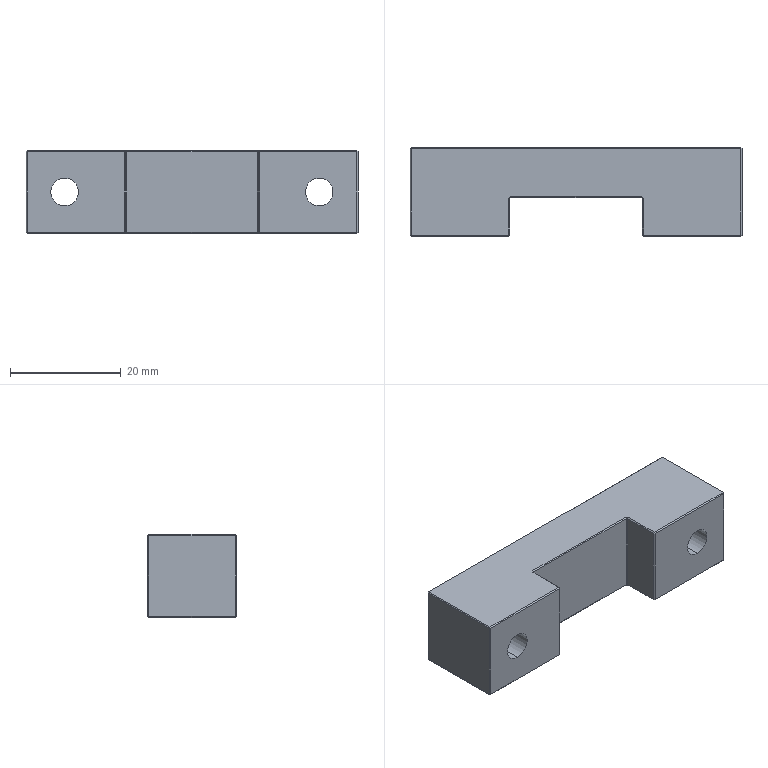Part | 1 solid | 58 faces | box 60 x 16 x 15 mm | volume 11243 mm3 | plane 50 | cone 4 | cylinder 4 | commonest cylinder face diameters 5 x4
STEP:
#1=CARTESIAN_POINT('',(22.997,-0.2,5.));
#2=VERTEX_POINT('',#1);
#3=CARTESIAN_POINT('',(22.997,-0.2,10.));
#4=VERTEX_POINT('',#3);
#5=CARTESIAN_POINT('',(22.997,-0.2,7.5));
#6=DIRECTION('',(0.,1.,0.));
#7=DIRECTION('',(0.,0.,-1.));
#8=AXIS2_PLACEMENT_3D('',#5,#6,#7);
#9=CIRCLE('',#8,2.5);
#10=EDGE_CURVE('',#2,#4,#9,.T.);
#11=ORIENTED_EDGE('',*,*,#10,.F.);
#12=CARTESIAN_POINT('',(22.997,0.,4.8));
#13=VERTEX_POINT('',#12);
#14=CARTESIAN_POINT('',(22.997,0.,4.8));
#15=DIRECTION('',(0.,0.7071,-0.7071));
#16=VECTOR('',#15,1000.);
#17=LINE('',#14,#16);
#18=EDGE_CURVE('',#2,#13,#17,.T.);
#19=ORIENTED_EDGE('',*,*,#18,.T.);
#20=CARTESIAN_POINT('',(22.997,0.,10.2));
#21=VERTEX_POINT('',#20);
#22=CARTESIAN_POINT('',(22.997,0.,7.5));
#23=DIRECTION('',(0.,-1.,0.));
#24=DIRECTION('',(1.,0.,0.));
#25=AXIS2_PLACEMENT_3D('',#22,#23,#24);
#26=CIRCLE('',#25,2.7);
#27=EDGE_CURVE('',#21,#13,#26,.T.);
#28=ORIENTED_EDGE('',*,*,#27,.F.);
#29=CARTESIAN_POINT('',(22.997,0.,10.2));
#30=DIRECTION('',(0.,0.7071,0.7071));
#31=VECTOR('',#30,1000.);
#32=LINE('',#29,#31);
#33=EDGE_CURVE('',#4,#21,#32,.T.);
#34=ORIENTED_EDGE('',*,*,#33,.F.);
#35=EDGE_LOOP('',(#11,#19,#28,#34));
#36=FACE_OUTER_BOUND('',#35,.T.);
#37=CARTESIAN_POINT('',(22.997,0.,7.5));
#38=DIRECTION('',(0.,1.,0.));
#39=DIRECTION('',(0.,0.,1.));
#40=AXIS2_PLACEMENT_3D('',#37,#38,#39);
#41=CONICAL_SURFACE('',#40,2.7,0.7854);
#42=ADVANCED_FACE('',(#36),#41,.F.);
#43=CARTESIAN_POINT('',(-23.003,-0.2,5.));
#44=VERTEX_POINT('',#43);
#45=CARTESIAN_POINT('',(-23.003,-0.2,10.));
#46=VERTEX_POINT('',#45);
#47=CARTESIAN_POINT('',(-23.003,-0.2,7.5));
#48=DIRECTION('',(0.,1.,0.));
#49=DIRECTION('',(0.,0.,-1.));
#50=AXIS2_PLACEMENT_3D('',#47,#48,#49);
#51=CIRCLE('',#50,2.5);
#52=EDGE_CURVE('',#44,#46,#51,.T.);
#53=ORIENTED_EDGE('',*,*,#52,.F.);
#54=CARTESIAN_POINT('',(-23.003,0.,4.8));
#55=VERTEX_POINT('',#54);
#56=CARTESIAN_POINT('',(-23.003,0.,4.8));
#57=DIRECTION('',(0.,0.7071,-0.7071));
#58=VECTOR('',#57,1000.);
#59=LINE('',#56,#58);
#60=EDGE_CURVE('',#44,#55,#59,.T.);
#61=ORIENTED_EDGE('',*,*,#60,.T.);
#62=CARTESIAN_POINT('',(-23.003,0.,10.2));
#63=VERTEX_POINT('',#62);
#64=CARTESIAN_POINT('',(-23.003,0.,7.5));
#65=DIRECTION('',(0.,-1.,0.));
#66=DIRECTION('',(1.,0.,0.));
#67=AXIS2_PLACEMENT_3D('',#64,#65,#66);
#68=CIRCLE('',#67,2.7);
#69=EDGE_CURVE('',#63,#55,#68,.T.);
#70=ORIENTED_EDGE('',*,*,#69,.F.);
#71=CARTESIAN_POINT('',(-23.003,0.,10.2));
#72=DIRECTION('',(0.,0.7071,0.7071));
#73=VECTOR('',#72,1000.);
#74=LINE('',#71,#73);
#75=EDGE_CURVE('',#46,#63,#74,.T.);
#76=ORIENTED_EDGE('',*,*,#75,.F.);
#77=EDGE_LOOP('',(#53,#61,#70,#76));
#78=FACE_OUTER_BOUND('',#77,.T.);
#79=CARTESIAN_POINT('',(-23.003,0.,7.5));
#80=DIRECTION('',(0.,1.,0.));
#81=DIRECTION('',(0.,0.,1.));
#82=AXIS2_PLACEMENT_3D('',#79,#80,#81);
#83=CONICAL_SURFACE('',#82,2.7,0.7854);
#84=ADVANCED_FACE('',(#78),#83,.F.);
#85=ORIENTED_EDGE('',*,*,#52,.T.);
#86=CARTESIAN_POINT('',(-23.003,-16.,10.));
#87=VERTEX_POINT('',#86);
#88=CARTESIAN_POINT('',(-23.003,-16.,10.));
#89=DIRECTION('',(0.,-1.,0.));
#90=VECTOR('',#89,1000.);
#91=LINE('',#88,#90);
#92=EDGE_CURVE('',#46,#87,#91,.T.);
#93=ORIENTED_EDGE('',*,*,#92,.T.);
#94=CARTESIAN_POINT('',(-23.003,-16.,5.));
#95=VERTEX_POINT('',#94);
#96=CARTESIAN_POINT('',(-23.003,-16.,7.5));
#97=DIRECTION('',(0.,-1.,0.));
#98=DIRECTION('',(0.,0.,-1.));
#99=AXIS2_PLACEMENT_3D('',#96,#97,#98);
#100=CIRCLE('',#99,2.5);
#101=EDGE_CURVE('',#87,#95,#100,.T.);
#102=ORIENTED_EDGE('',*,*,#101,.T.);
#103=CARTESIAN_POINT('',(-23.003,-16.,5.));
#104=DIRECTION('',(0.,-1.,0.));
#105=VECTOR('',#104,1000.);
#106=LINE('',#103,#105);
#107=EDGE_CURVE('',#44,#95,#106,.T.);
#108=ORIENTED_EDGE('',*,*,#107,.F.);
#109=EDGE_LOOP('',(#85,#93,#102,#108));
#110=FACE_OUTER_BOUND('',#109,.T.);
#111=CARTESIAN_POINT('',(-23.003,-16.,7.5));
#112=DIRECTION('',(0.,-1.,0.));
#113=DIRECTION('',(0.,0.,-1.));
#114=AXIS2_PLACEMENT_3D('',#111,#112,#113);
#115=CYLINDRICAL_SURFACE('',#114,2.5);
#116=ADVANCED_FACE('',(#110),#115,.F.);
#117=ORIENTED_EDGE('',*,*,#10,.T.);
#118=CARTESIAN_POINT('',(22.997,-16.,10.));
#119=VERTEX_POINT('',#118);
#120=CARTESIAN_POINT('',(22.997,-16.,10.));
#121=DIRECTION('',(0.,-1.,0.));
#122=VECTOR('',#121,1000.);
#123=LINE('',#120,#122);
#124=EDGE_CURVE('',#4,#119,#123,.T.);
#125=ORIENTED_EDGE('',*,*,#124,.T.);
#126=CARTESIAN_POINT('',(22.997,-16.,5.));
#127=VERTEX_POINT('',#126);
#128=CARTESIAN_POINT('',(22.997,-16.,7.5));
#129=DIRECTION('',(0.,-1.,0.));
#130=DIRECTION('',(0.,0.,-1.));
#131=AXIS2_PLACEMENT_3D('',#128,#129,#130);
#132=CIRCLE('',#131,2.5);
#133=EDGE_CURVE('',#119,#127,#132,.T.);
#134=ORIENTED_EDGE('',*,*,#133,.T.);
#135=CARTESIAN_POINT('',(22.997,-16.,5.));
#136=DIRECTION('',(0.,-1.,0.));
#137=VECTOR('',#136,1000.);
#138=LINE('',#135,#137);
#139=EDGE_CURVE('',#2,#127,#138,.T.);
#140=ORIENTED_EDGE('',*,*,#139,.F.);
#141=EDGE_LOOP('',(#117,#125,#134,#140));
#142=FACE_OUTER_BOUND('',#141,.T.);
#143=CARTESIAN_POINT('',(22.997,-16.,7.5));
#144=DIRECTION('',(0.,-1.,0.));
#145=DIRECTION('',(0.,0.,-1.));
#146=AXIS2_PLACEMENT_3D('',#143,#144,#145);
#147=CYLINDRICAL_SURFACE('',#146,2.5);
#148=ADVANCED_FACE('',(#142),#147,.F.);
#149=CARTESIAN_POINT('',(29.8,-0.2,0.));
#150=VERTEX_POINT('',#149);
#151=CARTESIAN_POINT('',(29.8,-15.8,0.));
#152=VERTEX_POINT('',#151);
#153=CARTESIAN_POINT('',(29.8,-16.,0.));
#154=DIRECTION('',(0.,-1.,0.));
#155=VECTOR('',#154,1000.);
#156=LINE('',#153,#155);
#157=EDGE_CURVE('',#150,#152,#156,.T.);
#158=ORIENTED_EDGE('',*,*,#157,.T.);
#159=CARTESIAN_POINT('',(12.2,-15.8,0.));
#160=VERTEX_POINT('',#159);
#161=CARTESIAN_POINT('',(12.,-15.8,0.));
#162=DIRECTION('',(-1.,0.,0.));
#163=VECTOR('',#162,1000.);
#164=LINE('',#161,#163);
#165=EDGE_CURVE('',#152,#160,#164,.T.);
#166=ORIENTED_EDGE('',*,*,#165,.T.);
#167=CARTESIAN_POINT('',(12.2,-9.2,0.));
#168=VERTEX_POINT('',#167);
#169=CARTESIAN_POINT('',(12.2,-9.,0.));
#170=DIRECTION('',(0.,1.,0.));
#171=VECTOR('',#170,1000.);
#172=LINE('',#169,#171);
#173=EDGE_CURVE('',#160,#168,#172,.T.);
#174=ORIENTED_EDGE('',*,*,#173,.T.);
#175=CARTESIAN_POINT('',(11.8,-8.8,0.));
#176=VERTEX_POINT('',#175);
#177=CARTESIAN_POINT('',(1.5,1.5,0.));
#178=DIRECTION('',(0.7071,-0.7071,0.));
#179=VECTOR('',#178,1000.);
#180=LINE('',#177,#179);
#181=EDGE_CURVE('',#176,#168,#180,.T.);
#182=ORIENTED_EDGE('',*,*,#181,.F.);
#183=CARTESIAN_POINT('',(-11.8,-8.8,0.));
#184=VERTEX_POINT('',#183);
#185=CARTESIAN_POINT('',(-12.,-8.8,0.));
#186=DIRECTION('',(-1.,0.,0.));
#187=VECTOR('',#186,1000.);
#188=LINE('',#185,#187);
#189=EDGE_CURVE('',#176,#184,#188,.T.);
#190=ORIENTED_EDGE('',*,*,#189,.T.);
#191=CARTESIAN_POINT('',(-12.2,-9.2,0.));
#192=VERTEX_POINT('',#191);
#193=CARTESIAN_POINT('',(-1.5,1.5,0.));
#194=DIRECTION('',(0.7071,0.7071,0.));
#195=VECTOR('',#194,1000.);
#196=LINE('',#193,#195);
#197=EDGE_CURVE('',#192,#184,#196,.T.);
#198=ORIENTED_EDGE('',*,*,#197,.F.);
#199=CARTESIAN_POINT('',(-12.2,-15.8,0.));
#200=VERTEX_POINT('',#199);
#201=CARTESIAN_POINT('',(-12.2,-16.,0.));
#202=DIRECTION('',(0.,-1.,0.));
#203=VECTOR('',#202,1000.);
#204=LINE('',#201,#203);
#205=EDGE_CURVE('',#192,#200,#204,.T.);
#206=ORIENTED_EDGE('',*,*,#205,.T.);
#207=CARTESIAN_POINT('',(-29.8,-15.8,0.));
#208=VERTEX_POINT('',#207);
#209=CARTESIAN_POINT('',(-30.,-15.8,0.));
#210=DIRECTION('',(-1.,0.,0.));
#211=VECTOR('',#210,1000.);
#212=LINE('',#209,#211);
#213=EDGE_CURVE('',#200,#208,#212,.T.);
#214=ORIENTED_EDGE('',*,*,#213,.T.);
#215=CARTESIAN_POINT('',(-29.8,-0.2,0.));
#216=VERTEX_POINT('',#215);
#217=CARTESIAN_POINT('',(-29.8,0.,0.));
#218=DIRECTION('',(0.,1.,0.));
#219=VECTOR('',#218,1000.);
#220=LINE('',#217,#219);
#221=EDGE_CURVE('',#208,#216,#220,.T.);
#222=ORIENTED_EDGE('',*,*,#221,.T.);
#223=CARTESIAN_POINT('',(30.,-0.2,0.));
#224=DIRECTION('',(1.,0.,0.));
#225=VECTOR('',#224,1000.);
#226=LINE('',#223,#225);
#227=EDGE_CURVE('',#216,#150,#226,.T.);
#228=ORIENTED_EDGE('',*,*,#227,.T.);
#229=EDGE_LOOP('',(#158,#166,#174,#182,#190,#198,#206,#214,#222,#228));
#230=FACE_OUTER_BOUND('',#229,.T.);
#231=CARTESIAN_POINT('',(0.,0.,0.));
#232=DIRECTION('',(0.,0.,-1.));
#233=DIRECTION('',(-1.,0.,0.));
#234=AXIS2_PLACEMENT_3D('',#231,#232,#233);
#235=PLANE('',#234);
#236=ADVANCED_FACE('',(#230),#235,.T.);
#237=CARTESIAN_POINT('',(12.2,-9.2,15.));
#238=VERTEX_POINT('',#237);
#239=CARTESIAN_POINT('',(12.2,-15.8,15.));
#240=VERTEX_POINT('',#239);
#241=CARTESIAN_POINT('',(12.2,0.,15.));
#242=DIRECTION('',(0.,-1.,0.));
#243=VECTOR('',#242,1000.);
#244=LINE('',#241,#243);
#245=EDGE_CURVE('',#238,#240,#244,.T.);
#246=ORIENTED_EDGE('',*,*,#245,.T.);
#247=CARTESIAN_POINT('',(29.8,-15.8,15.));
#248=VERTEX_POINT('',#247);
#249=CARTESIAN_POINT('',(0.,-15.8,15.));
#250=DIRECTION('',(1.,0.,0.));
#251=VECTOR('',#250,1000.);
#252=LINE('',#249,#251);
#253=EDGE_CURVE('',#240,#248,#252,.T.);
#254=ORIENTED_EDGE('',*,*,#253,.T.);
#255=CARTESIAN_POINT('',(29.8,-0.2,15.));
#256=VERTEX_POINT('',#255);
#257=CARTESIAN_POINT('',(29.8,0.,15.));
#258=DIRECTION('',(0.,1.,0.));
#259=VECTOR('',#258,1000.);
#260=LINE('',#257,#259);
#261=EDGE_CURVE('',#248,#256,#260,.T.);
#262=ORIENTED_EDGE('',*,*,#261,.T.);
#263=CARTESIAN_POINT('',(-29.8,-0.2,15.));
#264=VERTEX_POINT('',#263);
#265=CARTESIAN_POINT('',(0.,-0.2,15.));
#266=DIRECTION('',(-1.,0.,0.));
#267=VECTOR('',#266,1000.);
#268=LINE('',#265,#267);
#269=EDGE_CURVE('',#256,#264,#268,.T.);
#270=ORIENTED_EDGE('',*,*,#269,.T.);
#271=CARTESIAN_POINT('',(-29.8,-15.8,15.));
#272=VERTEX_POINT('',#271);
#273=CARTESIAN_POINT('',(-29.8,0.,15.));
#274=DIRECTION('',(0.,-1.,0.));
#275=VECTOR('',#274,1000.);
#276=LINE('',#273,#275);
#277=EDGE_CURVE('',#264,#272,#276,.T.);
#278=ORIENTED_EDGE('',*,*,#277,.T.);
#279=CARTESIAN_POINT('',(-12.2,-15.8,15.));
#280=VERTEX_POINT('',#279);
#281=CARTESIAN_POINT('',(0.,-15.8,15.));
#282=DIRECTION('',(1.,0.,0.));
#283=VECTOR('',#282,1000.);
#284=LINE('',#281,#283);
#285=EDGE_CURVE('',#272,#280,#284,.T.);
#286=ORIENTED_EDGE('',*,*,#285,.T.);
#287=CARTESIAN_POINT('',(-12.2,-9.2,15.));
#288=VERTEX_POINT('',#287);
#289=CARTESIAN_POINT('',(-12.2,0.,15.));
#290=DIRECTION('',(0.,1.,0.));
#291=VECTOR('',#290,1000.);
#292=LINE('',#289,#291);
#293=EDGE_CURVE('',#280,#288,#292,.T.);
#294=ORIENTED_EDGE('',*,*,#293,.T.);
#295=CARTESIAN_POINT('',(-11.8,-8.8,15.));
#296=VERTEX_POINT('',#295);
#297=CARTESIAN_POINT('',(-12.2,-9.2,15.));
#298=DIRECTION('',(-0.7071,-0.7071,0.));
#299=VECTOR('',#298,1000.);
#300=LINE('',#297,#299);
#301=EDGE_CURVE('',#296,#288,#300,.T.);
#302=ORIENTED_EDGE('',*,*,#301,.F.);
#303=CARTESIAN_POINT('',(11.8,-8.8,15.));
#304=VERTEX_POINT('',#303);
#305=CARTESIAN_POINT('',(0.,-8.8,15.));
#306=DIRECTION('',(1.,0.,0.));
#307=VECTOR('',#306,1000.);
#308=LINE('',#305,#307);
#309=EDGE_CURVE('',#296,#304,#308,.T.);
#310=ORIENTED_EDGE('',*,*,#309,.T.);
#311=CARTESIAN_POINT('',(11.8,-8.8,15.));
#312=DIRECTION('',(-0.7071,0.7071,0.));
#313=VECTOR('',#312,1000.);
#314=LINE('',#311,#313);
#315=EDGE_CURVE('',#238,#304,#314,.T.);
#316=ORIENTED_EDGE('',*,*,#315,.F.);
#317=EDGE_LOOP('',(#246,#254,#262,#270,#278,#286,#294,#302,#310,#316));
#318=FACE_OUTER_BOUND('',#317,.T.);
#319=CARTESIAN_POINT('',(0.,0.,15.));
#320=DIRECTION('',(0.,0.,-1.));
#321=DIRECTION('',(-1.,0.,0.));
#322=AXIS2_PLACEMENT_3D('',#319,#320,#321);
#323=PLANE('',#322);
#324=ADVANCED_FACE('',(#318),#323,.F.);
#325=CARTESIAN_POINT('',(-30.,-0.2,0.2));
#326=VERTEX_POINT('',#325);
#327=CARTESIAN_POINT('',(-30.,-15.8,0.2));
#328=VERTEX_POINT('',#327);
#329=CARTESIAN_POINT('',(-30.,-16.,0.2));
#330=DIRECTION('',(0.,-1.,0.));
#331=VECTOR('',#330,1000.);
#332=LINE('',#329,#331);
#333=EDGE_CURVE('',#326,#328,#332,.T.);
#334=ORIENTED_EDGE('',*,*,#333,.T.);
#335=CARTESIAN_POINT('',(-30.,-15.8,14.8));
#336=VERTEX_POINT('',#335);
#337=CARTESIAN_POINT('',(-30.,-15.8,15.));
#338=DIRECTION('',(0.,0.,1.));
#339=VECTOR('',#338,1000.);
#340=LINE('',#337,#339);
#341=EDGE_CURVE('',#328,#336,#340,.T.);
#342=ORIENTED_EDGE('',*,*,#341,.T.);
#343=CARTESIAN_POINT('',(-30.,-0.2,14.8));
#344=VERTEX_POINT('',#343);
#345=CARTESIAN_POINT('',(-30.,-16.,14.8));
#346=DIRECTION('',(0.,1.,0.));
#347=VECTOR('',#346,1000.);
#348=LINE('',#345,#347);
#349=EDGE_CURVE('',#336,#344,#348,.T.);
#350=ORIENTED_EDGE('',*,*,#349,.T.);
#351=CARTESIAN_POINT('',(-30.,-0.2,15.));
#352=DIRECTION('',(0.,0.,-1.));
#353=VECTOR('',#352,1000.);
#354=LINE('',#351,#353);
#355=EDGE_CURVE('',#344,#326,#354,.T.);
#356=ORIENTED_EDGE('',*,*,#355,.T.);
#357=EDGE_LOOP('',(#334,#342,#350,#356));
#358=FACE_OUTER_BOUND('',#357,.T.);
#359=CARTESIAN_POINT('',(-30.,-16.,15.));
#360=DIRECTION('',(1.,0.,0.));
#361=DIRECTION('',(0.,0.,-1.));
#362=AXIS2_PLACEMENT_3D('',#359,#360,#361);
#363=PLANE('',#362);
#364=ADVANCED_FACE('',(#358),#363,.F.);
#365=CARTESIAN_POINT('',(-23.003,-16.,7.5));
#366=DIRECTION('',(0.,-1.,0.));
#367=DIRECTION('',(0.,0.,-1.));
#368=AXIS2_PLACEMENT_3D('',#365,#366,#367);
#369=CIRCLE('',#368,2.5);
#370=EDGE_CURVE('',#95,#87,#369,.T.);
#371=ORIENTED_EDGE('',*,*,#370,.F.);
#372=ORIENTED_EDGE('',*,*,#101,.F.);
#373=EDGE_LOOP('',(#371,#372));
#374=FACE_BOUND('',#373,.T.);
#375=CARTESIAN_POINT('',(-12.2,-16.,0.2));
#376=VERTEX_POINT('',#375);
#377=CARTESIAN_POINT('',(-12.2,-16.,14.8));
#378=VERTEX_POINT('',#377);
#379=CARTESIAN_POINT('',(-12.2,-16.,15.));
#380=DIRECTION('',(0.,0.,1.));
#381=VECTOR('',#380,1000.);
#382=LINE('',#379,#381);
#383=EDGE_CURVE('',#376,#378,#382,.T.);
#384=ORIENTED_EDGE('',*,*,#383,.T.);
#385=CARTESIAN_POINT('',(-29.8,-16.,14.8));
#386=VERTEX_POINT('',#385);
#387=CARTESIAN_POINT('',(-12.,-16.,14.8));
#388=DIRECTION('',(-1.,0.,0.));
#389=VECTOR('',#388,1000.);
#390=LINE('',#387,#389);
#391=EDGE_CURVE('',#378,#386,#390,.T.);
#392=ORIENTED_EDGE('',*,*,#391,.T.);
#393=CARTESIAN_POINT('',(-29.8,-16.,0.2));
#394=VERTEX_POINT('',#393);
#395=CARTESIAN_POINT('',(-29.8,-16.,15.));
#396=DIRECTION('',(0.,0.,-1.));
#397=VECTOR('',#396,1000.);
#398=LINE('',#395,#397);
#399=EDGE_CURVE('',#386,#394,#398,.T.);
#400=ORIENTED_EDGE('',*,*,#399,.T.);
#401=CARTESIAN_POINT('',(-12.,-16.,0.2));
#402=DIRECTION('',(1.,0.,0.));
#403=VECTOR('',#402,1000.);
#404=LINE('',#401,#403);
#405=EDGE_CURVE('',#394,#376,#404,.T.);
#406=ORIENTED_EDGE('',*,*,#405,.T.);
#407=EDGE_LOOP('',(#384,#392,#400,#406));
#408=FACE_OUTER_BOUND('',#407,.T.);
#409=CARTESIAN_POINT('',(-12.,-16.,15.));
#410=DIRECTION('',(0.,1.,0.));
#411=DIRECTION('',(0.,0.,1.));
#412=AXIS2_PLACEMENT_3D('',#409,#410,#411);
#413=PLANE('',#412);
#414=ADVANCED_FACE('',(#374,#408),#413,.F.);
#415=CARTESIAN_POINT('',(-12.,-9.2,0.2));
#416=VERTEX_POINT('',#415);
#417=CARTESIAN_POINT('',(-12.,-9.2,14.8));
#418=VERTEX_POINT('',#417);
#419=CARTESIAN_POINT('',(-12.,-9.2,15.));
#420=DIRECTION('',(0.,0.,1.));
#421=VECTOR('',#420,1000.);
#422=LINE('',#419,#421);
#423=EDGE_CURVE('',#416,#418,#422,.T.);
#424=ORIENTED_EDGE('',*,*,#423,.T.);
#425=CARTESIAN_POINT('',(-12.,-15.8,14.8));
#426=VERTEX_POINT('',#425);
#427=CARTESIAN_POINT('',(-12.,-9.,14.8));
#428=DIRECTION('',(0.,-1.,0.));
#429=VECTOR('',#428,1000.);
#430=LINE('',#427,#429);
#431=EDGE_CURVE('',#418,#426,#430,.T.);
#432=ORIENTED_EDGE('',*,*,#431,.T.);
#433=CARTESIAN_POINT('',(-12.,-15.8,0.2));
#434=VERTEX_POINT('',#433);
#435=CARTESIAN_POINT('',(-12.,-15.8,15.));
#436=DIRECTION('',(0.,0.,-1.));
#437=VECTOR('',#436,1000.);
#438=LINE('',#435,#437);
#439=EDGE_CURVE('',#426,#434,#438,.T.);
#440=ORIENTED_EDGE('',*,*,#439,.T.);
#441=CARTESIAN_POINT('',(-12.,-9.,0.2));
#442=DIRECTION('',(0.,1.,0.));
#443=VECTOR('',#442,1000.);
#444=LINE('',#441,#443);
#445=EDGE_CURVE('',#434,#416,#444,.T.);
#446=ORIENTED_EDGE('',*,*,#445,.T.);
#447=EDGE_LOOP('',(#424,#432,#440,#446));
#448=FACE_OUTER_BOUND('',#447,.T.);
#449=CARTESIAN_POINT('',(-12.,-9.,15.));
#450=DIRECTION('',(-1.,0.,0.));
#451=DIRECTION('',(0.,-1.,0.));
#452=AXIS2_PLACEMENT_3D('',#449,#450,#451);
#453=PLANE('',#452);
#454=ADVANCED_FACE('',(#448),#453,.F.);
#455=CARTESIAN_POINT('',(11.8,-9.,0.2));
#456=VERTEX_POINT('',#455);
#457=CARTESIAN_POINT('',(11.8,-9.,14.8));
#458=VERTEX_POINT('',#457);
#459=CARTESIAN_POINT('',(11.8,-9.,15.));
#460=DIRECTION('',(0.,0.,1.));
#461=VECTOR('',#460,1000.);
#462=LINE('',#459,#461);
#463=EDGE_CURVE('',#456,#458,#462,.T.);
#464=ORIENTED_EDGE('',*,*,#463,.T.);
#465=CARTESIAN_POINT('',(-11.8,-9.,14.8));
#466=VERTEX_POINT('',#465);
#467=CARTESIAN_POINT('',(12.,-9.,14.8));
#468=DIRECTION('',(-1.,0.,0.));
#469=VECTOR('',#468,1000.);
#470=LINE('',#467,#469);
#471=EDGE_CURVE('',#458,#466,#470,.T.);
#472=ORIENTED_EDGE('',*,*,#471,.T.);
#473=CARTESIAN_POINT('',(-11.8,-9.,0.2));
#474=VERTEX_POINT('',#473);
#475=CARTESIAN_POINT('',(-11.8,-9.,0.));
#476=DIRECTION('',(0.,0.,-1.));
#477=VECTOR('',#476,1000.);
#478=LINE('',#475,#477);
#479=EDGE_CURVE('',#466,#474,#478,.T.);
#480=ORIENTED_EDGE('',*,*,#479,.T.);
#481=CARTESIAN_POINT('',(12.,-9.,0.2));
#482=DIRECTION('',(1.,0.,0.));
#483=VECTOR('',#482,1000.);
#484=LINE('',#481,#483);
#485=EDGE_CURVE('',#474,#456,#484,.T.);
#486=ORIENTED_EDGE('',*,*,#485,.T.);
#487=EDGE_LOOP('',(#464,#472,#480,#486));
#488=FACE_OUTER_BOUND('',#487,.T.);
#489=CARTESIAN_POINT('',(12.,-9.,15.));
#490=DIRECTION('',(0.,1.,0.));
#491=DIRECTION('',(-1.,0.,0.));
#492=AXIS2_PLACEMENT_3D('',#489,#490,#491);
#493=PLANE('',#492);
#494=ADVANCED_FACE('',(#488),#493,.F.);
#495=CARTESIAN_POINT('',(12.,-15.8,0.2));
#496=VERTEX_POINT('',#495);
#497=CARTESIAN_POINT('',(12.,-15.8,14.8));
#498=VERTEX_POINT('',#497);
#499=CARTESIAN_POINT('',(12.,-15.8,15.));
#500=DIRECTION('',(0.,0.,1.));
#501=VECTOR('',#500,1000.);
#502=LINE('',#499,#501);
#503=EDGE_CURVE('',#496,#498,#502,.T.);
#504=ORIENTED_EDGE('',*,*,#503,.T.);
#505=CARTESIAN_POINT('',(12.,-9.2,14.8));
#506=VERTEX_POINT('',#505);
#507=CARTESIAN_POINT('',(12.,-16.,14.8));
#508=DIRECTION('',(0.,1.,0.));
#509=VECTOR('',#508,1000.);
#510=LINE('',#507,#509);
#511=EDGE_CURVE('',#498,#506,#510,.T.);
#512=ORIENTED_EDGE('',*,*,#511,.T.);
#513=CARTESIAN_POINT('',(12.,-9.2,0.2));
#514=VERTEX_POINT('',#513);
#515=CARTESIAN_POINT('',(12.,-9.2,0.));
#516=DIRECTION('',(0.,0.,-1.));
#517=VECTOR('',#516,1000.);
#518=LINE('',#515,#517);
#519=EDGE_CURVE('',#506,#514,#518,.T.);
#520=ORIENTED_EDGE('',*,*,#519,.T.);
#521=CARTESIAN_POINT('',(12.,-16.,0.2));
#522=DIRECTION('',(0.,-1.,0.));
#523=VECTOR('',#522,1000.);
#524=LINE('',#521,#523);
#525=EDGE_CURVE('',#514,#496,#524,.T.);
#526=ORIENTED_EDGE('',*,*,#525,.T.);
#527=EDGE_LOOP('',(#504,#512,#520,#526));
#528=FACE_OUTER_BOUND('',#527,.T.);
#529=CARTESIAN_POINT('',(12.,-16.,15.));
#530=DIRECTION('',(1.,0.,0.));
#531=DIRECTION('',(0.,1.,0.));
#532=AXIS2_PLACEMENT_3D('',#529,#530,#531);
#533=PLANE('',#532);
#534=ADVANCED_FACE('',(#528),#533,.F.);
#535=CARTESIAN_POINT('',(22.997,-16.,7.5));
#536=DIRECTION('',(0.,-1.,0.));
#537=DIRECTION('',(0.,0.,-1.));
#538=AXIS2_PLACEMENT_3D('',#535,#536,#537);
#539=CIRCLE('',#538,2.5);
#540=EDGE_CURVE('',#127,#119,#539,.T.);
#541=ORIENTED_EDGE('',*,*,#540,.F.);
#542=ORIENTED_EDGE('',*,*,#133,.F.);
#543=EDGE_LOOP('',(#541,#542));
#544=FACE_BOUND('',#543,.T.);
#545=CARTESIAN_POINT('',(29.8,-16.,0.2));
#546=VERTEX_POINT('',#545);
#547=CARTESIAN_POINT('',(29.8,-16.,14.8));
#548=VERTEX_POINT('',#547);
#549=CARTESIAN_POINT('',(29.8,-16.,15.));
#550=DIRECTION('',(0.,0.,1.));
#551=VECTOR('',#550,1000.);
#552=LINE('',#549,#551);
#553=EDGE_CURVE('',#546,#548,#552,.T.);
#554=ORIENTED_EDGE('',*,*,#553,.T.);
#555=CARTESIAN_POINT('',(12.2,-16.,14.8));
#556=VERTEX_POINT('',#555);
#557=CARTESIAN_POINT('',(30.,-16.,14.8));
#558=DIRECTION('',(-1.,0.,0.));
#559=VECTOR('',#558,1000.);
#560=LINE('',#557,#559);
#561=EDGE_CURVE('',#548,#556,#560,.T.);
#562=ORIENTED_EDGE('',*,*,#561,.T.);
#563=CARTESIAN_POINT('',(12.2,-16.,0.2));
#564=VERTEX_POINT('',#563);
#565=CARTESIAN_POINT('',(12.2,-16.,15.));
#566=DIRECTION('',(0.,0.,-1.));
#567=VECTOR('',#566,1000.);
#568=LINE('',#565,#567);
#569=EDGE_CURVE('',#556,#564,#568,.T.);
#570=ORIENTED_EDGE('',*,*,#569,.T.);
#571=CARTESIAN_POINT('',(30.,-16.,0.2));
#572=DIRECTION('',(1.,0.,0.));
#573=VECTOR('',#572,1000.);
#574=LINE('',#571,#573);
#575=EDGE_CURVE('',#564,#546,#574,.T.);
#576=ORIENTED_EDGE('',*,*,#575,.T.);
#577=EDGE_LOOP('',(#554,#562,#570,#576));
#578=FACE_OUTER_BOUND('',#577,.T.);
#579=CARTESIAN_POINT('',(30.,-16.,15.));
#580=DIRECTION('',(0.,1.,0.));
#581=DIRECTION('',(-1.,0.,0.));
#582=AXIS2_PLACEMENT_3D('',#579,#580,#581);
#583=PLANE('',#582);
#584=ADVANCED_FACE('',(#544,#578),#583,.F.);
#585=CARTESIAN_POINT('',(30.,-0.2,0.2));
#586=VERTEX_POINT('',#585);
#587=CARTESIAN_POINT('',(30.,-0.2,14.8));
#588=VERTEX_POINT('',#587);
#589=CARTESIAN_POINT('',(30.,-0.2,15.));
#590=DIRECTION('',(0.,0.,1.));
#591=VECTOR('',#590,1000.);
#592=LINE('',#589,#591);
#593=EDGE_CURVE('',#586,#588,#592,.T.);
#594=ORIENTED_EDGE('',*,*,#593,.T.);
#595=CARTESIAN_POINT('',(30.,-15.8,14.8));
#596=VERTEX_POINT('',#595);
#597=CARTESIAN_POINT('',(30.,0.,14.8));
#598=DIRECTION('',(0.,-1.,0.));
#599=VECTOR('',#598,1000.);
#600=LINE('',#597,#599);
#601=EDGE_CURVE('',#588,#596,#600,.T.);
#602=ORIENTED_EDGE('',*,*,#601,.T.);
#603=CARTESIAN_POINT('',(30.,-15.8,0.2));
#604=VERTEX_POINT('',#603);
#605=CARTESIAN_POINT('',(30.,-15.8,15.));
#606=DIRECTION('',(0.,0.,-1.));
#607=VECTOR('',#606,1000.);
#608=LINE('',#605,#607);
#609=EDGE_CURVE('',#596,#604,#608,.T.);
#610=ORIENTED_EDGE('',*,*,#609,.T.);
#611=CARTESIAN_POINT('',(30.,0.,0.2));
#612=DIRECTION('',(0.,1.,0.));
#613=VECTOR('',#612,1000.);
#614=LINE('',#611,#613);
#615=EDGE_CURVE('',#604,#586,#614,.T.);
#616=ORIENTED_EDGE('',*,*,#615,.T.);
#617=EDGE_LOOP('',(#594,#602,#610,#616));
#618=FACE_OUTER_BOUND('',#617,.T.);
#619=CARTESIAN_POINT('',(30.,0.,15.));
#620=DIRECTION('',(-1.,0.,0.));
#621=DIRECTION('',(0.,0.,1.));
#622=AXIS2_PLACEMENT_3D('',#619,#620,#621);
#623=PLANE('',#622);
#624=ADVANCED_FACE('',(#618),#623,.F.);
#625=ORIENTED_EDGE('',*,*,#69,.T.);
#626=CARTESIAN_POINT('',(-23.003,0.,7.5));
#627=DIRECTION('',(0.,-1.,0.));
#628=DIRECTION('',(1.,0.,0.));
#629=AXIS2_PLACEMENT_3D('',#626,#627,#628);
#630=CIRCLE('',#629,2.7);
#631=EDGE_CURVE('',#55,#63,#630,.T.);
#632=ORIENTED_EDGE('',*,*,#631,.T.);
#633=EDGE_LOOP('',(#625,#632));
#634=FACE_BOUND('',#633,.T.);
#635=ORIENTED_EDGE('',*,*,#27,.T.);
#636=CARTESIAN_POINT('',(22.997,0.,7.5));
#637=DIRECTION('',(0.,-1.,0.));
#638=DIRECTION('',(1.,0.,0.));
#639=AXIS2_PLACEMENT_3D('',#636,#637,#638);
#640=CIRCLE('',#639,2.7);
#641=EDGE_CURVE('',#13,#21,#640,.T.);
#642=ORIENTED_EDGE('',*,*,#641,.T.);
#643=EDGE_LOOP('',(#635,#642));
#644=FACE_BOUND('',#643,.T.);
#645=CARTESIAN_POINT('',(-29.8,0.,14.8));
#646=VERTEX_POINT('',#645);
#647=CARTESIAN_POINT('',(29.8,0.,14.8));
#648=VERTEX_POINT('',#647);
#649=CARTESIAN_POINT('',(-30.,0.,14.8));
#650=DIRECTION('',(1.,0.,0.));
#651=VECTOR('',#650,1000.);
#652=LINE('',#649,#651);
#653=EDGE_CURVE('',#646,#648,#652,.T.);
#654=ORIENTED_EDGE('',*,*,#653,.T.);
#655=CARTESIAN_POINT('',(29.8,0.,0.2));
#656=VERTEX_POINT('',#655);
#657=CARTESIAN_POINT('',(29.8,0.,15.));
#658=DIRECTION('',(0.,0.,-1.));
#659=VECTOR('',#658,1000.);
#660=LINE('',#657,#659);
#661=EDGE_CURVE('',#648,#656,#660,.T.);
#662=ORIENTED_EDGE('',*,*,#661,.T.);
#663=CARTESIAN_POINT('',(-29.8,0.,0.2));
#664=VERTEX_POINT('',#663);
#665=CARTESIAN_POINT('',(-30.,0.,0.2));
#666=DIRECTION('',(-1.,0.,0.));
#667=VECTOR('',#666,1000.);
#668=LINE('',#665,#667);
#669=EDGE_CURVE('',#656,#664,#668,.T.);
#670=ORIENTED_EDGE('',*,*,#669,.T.);
#671=CARTESIAN_POINT('',(-29.8,0.,15.));
#672=DIRECTION('',(0.,0.,1.));
#673=VECTOR('',#672,1000.);
#674=LINE('',#671,#673);
#675=EDGE_CURVE('',#664,#646,#674,.T.);
#676=ORIENTED_EDGE('',*,*,#675,.T.);
#677=EDGE_LOOP('',(#654,#662,#670,#676));
#678=FACE_OUTER_BOUND('',#677,.T.);
#679=CARTESIAN_POINT('',(-30.,0.,15.));
#680=DIRECTION('',(0.,-1.,0.));
#681=DIRECTION('',(1.,0.,0.));
#682=AXIS2_PLACEMENT_3D('',#679,#680,#681);
#683=PLANE('',#682);
#684=ADVANCED_FACE('',(#634,#644,#678),#683,.F.);
#685=CARTESIAN_POINT('',(12.,-15.8,14.8));
#686=DIRECTION('',(0.7071,-0.7071,0.));
#687=VECTOR('',#686,1000.);
#688=LINE('',#685,#687);
#689=EDGE_CURVE('',#498,#556,#688,.T.);
#690=ORIENTED_EDGE('',*,*,#689,.F.);
#691=ORIENTED_EDGE('',*,*,#503,.F.);
#692=CARTESIAN_POINT('',(12.2,-16.,0.2));
#693=DIRECTION('',(-0.7071,0.7071,0.));
#694=VECTOR('',#693,1000.);
#695=LINE('',#692,#694);
#696=EDGE_CURVE('',#564,#496,#695,.T.);
#697=ORIENTED_EDGE('',*,*,#696,.F.);
#698=ORIENTED_EDGE('',*,*,#569,.F.);
#699=EDGE_LOOP('',(#690,#691,#697,#698));
#700=FACE_OUTER_BOUND('',#699,.T.);
#701=CARTESIAN_POINT('',(12.2,-16.,15.));
#702=DIRECTION('',(0.7071,0.7071,0.));
#703=DIRECTION('',(0.,0.,-1.));
#704=AXIS2_PLACEMENT_3D('',#701,#702,#703);
#705=PLANE('',#704);
#706=ADVANCED_FACE('',(#700),#705,.F.);
#707=CARTESIAN_POINT('',(12.,-15.8,14.8));
#708=DIRECTION('',(0.7071,0.,0.7071));
#709=VECTOR('',#708,1000.);
#710=LINE('',#707,#709);
#711=EDGE_CURVE('',#498,#240,#710,.T.);
#712=ORIENTED_EDGE('',*,*,#711,.F.);
#713=ORIENTED_EDGE('',*,*,#689,.T.);
#714=CARTESIAN_POINT('',(12.2,-15.9,14.9));
#715=DIRECTION('',(0.,-0.7071,-0.7071));
#716=VECTOR('',#715,1000.);
#717=LINE('',#714,#716);
#718=EDGE_CURVE('',#240,#556,#717,.T.);
#719=ORIENTED_EDGE('',*,*,#718,.F.);
#720=EDGE_LOOP('',(#712,#713,#719));
#721=FACE_OUTER_BOUND('',#720,.T.);
#722=CARTESIAN_POINT('',(12.,-15.8,14.8));
#723=DIRECTION('',(-0.5774,-0.5774,0.5774));
#724=DIRECTION('',(0.7071,-0.7071,0.));
#725=AXIS2_PLACEMENT_3D('',#722,#723,#724);
#726=PLANE('',#725);
#727=ADVANCED_FACE('',(#721),#726,.T.);
#728=CARTESIAN_POINT('',(12.2,-16.,0.2));
#729=DIRECTION('',(0.,0.7071,-0.7071));
#730=VECTOR('',#729,1000.);
#731=LINE('',#728,#730);
#732=EDGE_CURVE('',#564,#160,#731,.T.);
#733=ORIENTED_EDGE('',*,*,#732,.F.);
#734=ORIENTED_EDGE('',*,*,#696,.T.);
#735=CARTESIAN_POINT('',(12.1,-15.8,0.1));
#736=DIRECTION('',(-0.7071,0.,0.7071));
#737=VECTOR('',#736,1000.);
#738=LINE('',#735,#737);
#739=EDGE_CURVE('',#160,#496,#738,.T.);
#740=ORIENTED_EDGE('',*,*,#739,.F.);
#741=EDGE_LOOP('',(#733,#734,#740));
#742=FACE_OUTER_BOUND('',#741,.T.);
#743=CARTESIAN_POINT('',(12.2,-16.,0.2));
#744=DIRECTION('',(-0.5774,-0.5774,-0.5774));
#745=DIRECTION('',(-0.7071,0.,0.7071));
#746=AXIS2_PLACEMENT_3D('',#743,#744,#745);
#747=PLANE('',#746);
#748=ADVANCED_FACE('',(#742),#747,.T.);
#749=ORIENTED_EDGE('',*,*,#718,.T.);
#750=ORIENTED_EDGE('',*,*,#561,.F.);
#751=CARTESIAN_POINT('',(29.8,-16.,14.8));
#752=DIRECTION('',(0.,-0.7071,-0.7071));
#753=VECTOR('',#752,1000.);
#754=LINE('',#751,#753);
#755=EDGE_CURVE('',#248,#548,#754,.T.);
#756=ORIENTED_EDGE('',*,*,#755,.F.);
#757=ORIENTED_EDGE('',*,*,#253,.F.);
#758=EDGE_LOOP('',(#749,#750,#756,#757));
#759=FACE_OUTER_BOUND('',#758,.T.);
#760=CARTESIAN_POINT('',(0.,-15.8,15.));
#761=DIRECTION('',(0.,0.7071,-0.7071));
#762=DIRECTION('',(1.,0.,0.));
#763=AXIS2_PLACEMENT_3D('',#760,#761,#762);
#764=PLANE('',#763);
#765=ADVANCED_FACE('',(#759),#764,.F.);
#766=ORIENTED_EDGE('',*,*,#711,.T.);
#767=ORIENTED_EDGE('',*,*,#245,.F.);
#768=CARTESIAN_POINT('',(12.,-9.2,14.8));
#769=DIRECTION('',(0.7071,0.,0.7071));
#770=VECTOR('',#769,1000.);
#771=LINE('',#768,#770);
#772=EDGE_CURVE('',#506,#238,#771,.T.);
#773=ORIENTED_EDGE('',*,*,#772,.F.);
#774=ORIENTED_EDGE('',*,*,#511,.F.);
#775=EDGE_LOOP('',(#766,#767,#773,#774));
#776=FACE_OUTER_BOUND('',#775,.T.);
#777=CARTESIAN_POINT('',(12.2,0.,15.));
#778=DIRECTION('',(0.7071,0.,-0.7071));
#779=DIRECTION('',(0.,-1.,0.));
#780=AXIS2_PLACEMENT_3D('',#777,#778,#779);
#781=PLANE('',#780);
#782=ADVANCED_FACE('',(#776),#781,.F.);
#783=CARTESIAN_POINT('',(12.,-9.2,0.2));
#784=DIRECTION('',(-0.7071,0.7071,0.));
#785=VECTOR('',#784,1000.);
#786=LINE('',#783,#785);
#787=EDGE_CURVE('',#514,#456,#786,.T.);
#788=ORIENTED_EDGE('',*,*,#787,.F.);
#789=ORIENTED_EDGE('',*,*,#519,.F.);
#790=CARTESIAN_POINT('',(11.8,-9.,14.8));
#791=DIRECTION('',(0.7071,-0.7071,0.));
#792=VECTOR('',#791,1000.);
#793=LINE('',#790,#792);
#794=EDGE_CURVE('',#458,#506,#793,.T.);
#795=ORIENTED_EDGE('',*,*,#794,.F.);
#796=ORIENTED_EDGE('',*,*,#463,.F.);
#797=EDGE_LOOP('',(#788,#789,#795,#796));
#798=FACE_OUTER_BOUND('',#797,.T.);
#799=CARTESIAN_POINT('',(12.,-9.2,15.));
#800=DIRECTION('',(-0.7071,-0.7071,0.));
#801=DIRECTION('',(0.,0.,1.));
#802=AXIS2_PLACEMENT_3D('',#799,#800,#801);
#803=PLANE('',#802);
#804=ADVANCED_FACE('',(#798),#803,.T.);
#805=ORIENTED_EDGE('',*,*,#739,.T.);
#806=ORIENTED_EDGE('',*,*,#525,.F.);
#807=CARTESIAN_POINT('',(12.2,-9.2,0.));
#808=DIRECTION('',(-0.7071,0.,0.7071));
#809=VECTOR('',#808,1000.);
#810=LINE('',#807,#809);
#811=EDGE_CURVE('',#168,#514,#810,.T.);
#812=ORIENTED_EDGE('',*,*,#811,.F.);
#813=ORIENTED_EDGE('',*,*,#173,.F.);
#814=EDGE_LOOP('',(#805,#806,#812,#813));
#815=FACE_OUTER_BOUND('',#814,.T.);
#816=CARTESIAN_POINT('',(12.,-16.,0.2));
#817=DIRECTION('',(-0.7071,0.,-0.7071));
#818=DIRECTION('',(0.,1.,0.));
#819=AXIS2_PLACEMENT_3D('',#816,#817,#818);
#820=PLANE('',#819);
#821=ADVANCED_FACE('',(#815),#820,.T.);
#822=ORIENTED_EDGE('',*,*,#732,.T.);
#823=ORIENTED_EDGE('',*,*,#165,.F.);
#824=CARTESIAN_POINT('',(29.8,-15.9,0.1));
#825=DIRECTION('',(0.,0.7071,-0.7071));
#826=VECTOR('',#825,1000.);
#827=LINE('',#824,#826);
#828=EDGE_CURVE('',#546,#152,#827,.T.);
#829=ORIENTED_EDGE('',*,*,#828,.F.);
#830=ORIENTED_EDGE('',*,*,#575,.F.);
#831=EDGE_LOOP('',(#822,#823,#829,#830));
#832=FACE_OUTER_BOUND('',#831,.T.);
#833=CARTESIAN_POINT('',(30.,-16.,0.2));
#834=DIRECTION('',(0.,-0.7071,-0.7071));
#835=DIRECTION('',(-1.,0.,0.));
#836=AXIS2_PLACEMENT_3D('',#833,#834,#835);
#837=PLANE('',#836);
#838=ADVANCED_FACE('',(#832),#837,.T.);
#839=CARTESIAN_POINT('',(29.8,-16.,14.8));
#840=DIRECTION('',(0.7071,0.7071,0.));
#841=VECTOR('',#840,1000.);
#842=LINE('',#839,#841);
#843=EDGE_CURVE('',#548,#596,#842,.T.);
#844=ORIENTED_EDGE('',*,*,#843,.F.);
#845=ORIENTED_EDGE('',*,*,#553,.F.);
#846=CARTESIAN_POINT('',(30.,-15.8,0.2));
#847=DIRECTION('',(-0.7071,-0.7071,0.));
#848=VECTOR('',#847,1000.);
#849=LINE('',#846,#848);
#850=EDGE_CURVE('',#604,#546,#849,.T.);
#851=ORIENTED_EDGE('',*,*,#850,.F.);
#852=ORIENTED_EDGE('',*,*,#609,.F.);
#853=EDGE_LOOP('',(#844,#845,#851,#852));
#854=FACE_OUTER_BOUND('',#853,.T.);
#855=CARTESIAN_POINT('',(30.,-15.8,15.));
#856=DIRECTION('',(-0.7071,0.7071,0.));
#857=DIRECTION('',(0.,0.,-1.));
#858=AXIS2_PLACEMENT_3D('',#855,#856,#857);
#859=PLANE('',#858);
#860=ADVANCED_FACE('',(#854),#859,.F.);
#861=ORIENTED_EDGE('',*,*,#755,.T.);
#862=ORIENTED_EDGE('',*,*,#843,.T.);
#863=CARTESIAN_POINT('',(29.9,-15.8,14.9));
#864=DIRECTION('',(0.7071,0.,-0.7071));
#865=VECTOR('',#864,1000.);
#866=LINE('',#863,#865);
#867=EDGE_CURVE('',#248,#596,#866,.T.);
#868=ORIENTED_EDGE('',*,*,#867,.F.);
#869=EDGE_LOOP('',(#861,#862,#868));
#870=FACE_OUTER_BOUND('',#869,.T.);
#871=CARTESIAN_POINT('',(29.8,-16.,14.8));
#872=DIRECTION('',(0.5774,-0.5774,0.5774));
#873=DIRECTION('',(0.7071,0.7071,0.));
#874=AXIS2_PLACEMENT_3D('',#871,#872,#873);
#875=PLANE('',#874);
#876=ADVANCED_FACE('',(#870),#875,.T.);
#877=ORIENTED_EDGE('',*,*,#772,.T.);
#878=ORIENTED_EDGE('',*,*,#315,.T.);
#879=CARTESIAN_POINT('',(11.8,-8.8,15.));
#880=DIRECTION('',(0.,0.7071,0.7071));
#881=VECTOR('',#880,1000.);
#882=LINE('',#879,#881);
#883=EDGE_CURVE('',#458,#304,#882,.T.);
#884=ORIENTED_EDGE('',*,*,#883,.F.);
#885=ORIENTED_EDGE('',*,*,#794,.T.);
#886=EDGE_LOOP('',(#877,#878,#884,#885));
#887=FACE_OUTER_BOUND('',#886,.T.);
#888=CARTESIAN_POINT('',(11.8,-9.,14.8));
#889=DIRECTION('',(-0.5774,-0.5774,0.5774));
#890=DIRECTION('',(0.7071,-0.7071,0.));
#891=AXIS2_PLACEMENT_3D('',#888,#889,#890);
#892=PLANE('',#891);
#893=ADVANCED_FACE('',(#887),#892,.T.);
#894=ORIENTED_EDGE('',*,*,#811,.T.);
#895=ORIENTED_EDGE('',*,*,#787,.T.);
#896=CARTESIAN_POINT('',(11.8,-9.,0.2));
#897=DIRECTION('',(0.,-0.7071,0.7071));
#898=VECTOR('',#897,1000.);
#899=LINE('',#896,#898);
#900=EDGE_CURVE('',#176,#456,#899,.T.);
#901=ORIENTED_EDGE('',*,*,#900,.F.);
#902=ORIENTED_EDGE('',*,*,#181,.T.);
#903=EDGE_LOOP('',(#894,#895,#901,#902));
#904=FACE_OUTER_BOUND('',#903,.T.);
#905=CARTESIAN_POINT('',(12.,-9.2,0.2));
#906=DIRECTION('',(-0.5774,-0.5774,-0.5774));
#907=DIRECTION('',(0.,0.7071,-0.7071));
#908=AXIS2_PLACEMENT_3D('',#905,#906,#907);
#909=PLANE('',#908);
#910=ADVANCED_FACE('',(#904),#909,.T.);
#911=ORIENTED_EDGE('',*,*,#850,.T.);
#912=ORIENTED_EDGE('',*,*,#828,.T.);
#913=CARTESIAN_POINT('',(30.,-15.8,0.2));
#914=DIRECTION('',(-0.7071,0.,-0.7071));
#915=VECTOR('',#914,1000.);
#916=LINE('',#913,#915);
#917=EDGE_CURVE('',#604,#152,#916,.T.);
#918=ORIENTED_EDGE('',*,*,#917,.F.);
#919=EDGE_LOOP('',(#911,#912,#918));
#920=FACE_OUTER_BOUND('',#919,.T.);
#921=CARTESIAN_POINT('',(30.,-15.8,0.2));
#922=DIRECTION('',(0.5774,-0.5774,-0.5774));
#923=DIRECTION('',(0.,0.7071,-0.7071));
#924=AXIS2_PLACEMENT_3D('',#921,#922,#923);
#925=PLANE('',#924);
#926=ADVANCED_FACE('',(#920),#925,.T.);
#927=ORIENTED_EDGE('',*,*,#867,.T.);
#928=ORIENTED_EDGE('',*,*,#601,.F.);
#929=CARTESIAN_POINT('',(30.,-0.2,14.8));
#930=DIRECTION('',(0.7071,0.,-0.7071));
#931=VECTOR('',#930,1000.);
#932=LINE('',#929,#931);
#933=EDGE_CURVE('',#256,#588,#932,.T.);
#934=ORIENTED_EDGE('',*,*,#933,.F.);
#935=ORIENTED_EDGE('',*,*,#261,.F.);
#936=EDGE_LOOP('',(#927,#928,#934,#935));
#937=FACE_OUTER_BOUND('',#936,.T.);
#938=CARTESIAN_POINT('',(29.8,0.,15.));
#939=DIRECTION('',(-0.7071,0.,-0.7071));
#940=DIRECTION('',(0.,1.,0.));
#941=AXIS2_PLACEMENT_3D('',#938,#939,#940);
#942=PLANE('',#941);
#943=ADVANCED_FACE('',(#937),#942,.F.);
#944=ORIENTED_EDGE('',*,*,#883,.T.);
#945=ORIENTED_EDGE('',*,*,#309,.F.);
#946=CARTESIAN_POINT('',(-11.8,-9.,14.8));
#947=DIRECTION('',(0.,0.7071,0.7071));
#948=VECTOR('',#947,1000.);
#949=LINE('',#946,#948);
#950=EDGE_CURVE('',#466,#296,#949,.T.);
#951=ORIENTED_EDGE('',*,*,#950,.F.);
#952=ORIENTED_EDGE('',*,*,#471,.F.);
#953=EDGE_LOOP('',(#944,#945,#951,#952));
#954=FACE_OUTER_BOUND('',#953,.T.);
#955=CARTESIAN_POINT('',(0.,-8.8,15.));
#956=DIRECTION('',(0.,0.7071,-0.7071));
#957=DIRECTION('',(1.,0.,0.));
#958=AXIS2_PLACEMENT_3D('',#955,#956,#957);
#959=PLANE('',#958);
#960=ADVANCED_FACE('',(#954),#959,.F.);
#961=CARTESIAN_POINT('',(-11.8,-9.,0.2));
#962=DIRECTION('',(-0.7071,-0.7071,0.));
#963=VECTOR('',#962,1000.);
#964=LINE('',#961,#963);
#965=EDGE_CURVE('',#474,#416,#964,.T.);
#966=ORIENTED_EDGE('',*,*,#965,.F.);
#967=ORIENTED_EDGE('',*,*,#479,.F.);
#968=CARTESIAN_POINT('',(-12.,-9.2,14.8));
#969=DIRECTION('',(0.7071,0.7071,0.));
#970=VECTOR('',#969,1000.);
#971=LINE('',#968,#970);
#972=EDGE_CURVE('',#418,#466,#971,.T.);
#973=ORIENTED_EDGE('',*,*,#972,.F.);
#974=ORIENTED_EDGE('',*,*,#423,.F.);
#975=EDGE_LOOP('',(#966,#967,#973,#974));
#976=FACE_OUTER_BOUND('',#975,.T.);
#977=CARTESIAN_POINT('',(-11.8,-9.,15.));
#978=DIRECTION('',(0.7071,-0.7071,0.));
#979=DIRECTION('',(0.,0.,1.));
#980=AXIS2_PLACEMENT_3D('',#977,#978,#979);
#981=PLANE('',#980);
#982=ADVANCED_FACE('',(#976),#981,.T.);
#983=ORIENTED_EDGE('',*,*,#900,.T.);
#984=ORIENTED_EDGE('',*,*,#485,.F.);
#985=CARTESIAN_POINT('',(-11.8,-8.8,0.));
#986=DIRECTION('',(0.,-0.7071,0.7071));
#987=VECTOR('',#986,1000.);
#988=LINE('',#985,#987);
#989=EDGE_CURVE('',#184,#474,#988,.T.);
#990=ORIENTED_EDGE('',*,*,#989,.F.);
#991=ORIENTED_EDGE('',*,*,#189,.F.);
#992=EDGE_LOOP('',(#983,#984,#990,#991));
#993=FACE_OUTER_BOUND('',#992,.T.);
#994=CARTESIAN_POINT('',(12.,-9.,0.2));
#995=DIRECTION('',(0.,-0.7071,-0.7071));
#996=DIRECTION('',(-1.,0.,0.));
#997=AXIS2_PLACEMENT_3D('',#994,#995,#996);
#998=PLANE('',#997);
#999=ADVANCED_FACE('',(#993),#998,.T.);
#1000=ORIENTED_EDGE('',*,*,#917,.T.);
#1001=ORIENTED_EDGE('',*,*,#157,.F.);
#1002=CARTESIAN_POINT('',(29.9,-0.2,0.1));
#1003=DIRECTION('',(-0.7071,0.,-0.7071));
#1004=VECTOR('',#1003,1000.);
#1005=LINE('',#1002,#1004);
#1006=EDGE_CURVE('',#586,#150,#1005,.T.);
#1007=ORIENTED_EDGE('',*,*,#1006,.F.);
#1008=ORIENTED_EDGE('',*,*,#615,.F.);
#1009=EDGE_LOOP('',(#1000,#1001,#1007,#1008));
#1010=FACE_OUTER_BOUND('',#1009,.T.);
#1011=CARTESIAN_POINT('',(30.,0.,0.2));
#1012=DIRECTION('',(0.7071,0.,-0.7071));
#1013=DIRECTION('',(0.,-1.,0.));
#1014=AXIS2_PLACEMENT_3D('',#1011,#1012,#1013);
#1015=PLANE('',#1014);
#1016=ADVANCED_FACE('',(#1010),#1015,.T.);
#1017=CARTESIAN_POINT('',(30.,-0.2,14.8));
#1018=DIRECTION('',(-0.7071,0.7071,0.));
#1019=VECTOR('',#1018,1000.);
#1020=LINE('',#1017,#1019);
#1021=EDGE_CURVE('',#588,#648,#1020,.T.);
#1022=ORIENTED_EDGE('',*,*,#1021,.F.);
#1023=ORIENTED_EDGE('',*,*,#593,.F.);
#1024=CARTESIAN_POINT('',(29.8,0.,0.2));
#1025=DIRECTION('',(0.7071,-0.7071,0.));
#1026=VECTOR('',#1025,1000.);
#1027=LINE('',#1024,#1026);
#1028=EDGE_CURVE('',#656,#586,#1027,.T.);
#1029=ORIENTED_EDGE('',*,*,#1028,.F.);
#1030=ORIENTED_EDGE('',*,*,#661,.F.);
#1031=EDGE_LOOP('',(#1022,#1023,#1029,#1030));
#1032=FACE_OUTER_BOUND('',#1031,.T.);
#1033=CARTESIAN_POINT('',(29.8,0.,15.));
#1034=DIRECTION('',(-0.7071,-0.7071,0.));
#1035=DIRECTION('',(0.,0.,-1.));
#1036=AXIS2_PLACEMENT_3D('',#1033,#1034,#1035);
#1037=PLANE('',#1036);
#1038=ADVANCED_FACE('',(#1032),#1037,.F.);
#1039=ORIENTED_EDGE('',*,*,#933,.T.);
#1040=ORIENTED_EDGE('',*,*,#1021,.T.);
#1041=CARTESIAN_POINT('',(29.8,-0.1,14.9));
#1042=DIRECTION('',(0.,0.7071,-0.7071));
#1043=VECTOR('',#1042,1000.);
#1044=LINE('',#1041,#1043);
#1045=EDGE_CURVE('',#256,#648,#1044,.T.);
#1046=ORIENTED_EDGE('',*,*,#1045,.F.);
#1047=EDGE_LOOP('',(#1039,#1040,#1046));
#1048=FACE_OUTER_BOUND('',#1047,.T.);
#1049=CARTESIAN_POINT('',(30.,-0.2,14.8));
#1050=DIRECTION('',(0.5774,0.5774,0.5774));
#1051=DIRECTION('',(-0.7071,0.7071,0.));
#1052=AXIS2_PLACEMENT_3D('',#1049,#1050,#1051);
#1053=PLANE('',#1052);
#1054=ADVANCED_FACE('',(#1048),#1053,.T.);
#1055=ORIENTED_EDGE('',*,*,#950,.T.);
#1056=ORIENTED_EDGE('',*,*,#301,.T.);
#1057=CARTESIAN_POINT('',(-12.2,-9.2,15.));
#1058=DIRECTION('',(-0.7071,0.,0.7071));
#1059=VECTOR('',#1058,1000.);
#1060=LINE('',#1057,#1059);
#1061=EDGE_CURVE('',#418,#288,#1060,.T.);
#1062=ORIENTED_EDGE('',*,*,#1061,.F.);
#1063=ORIENTED_EDGE('',*,*,#972,.T.);
#1064=EDGE_LOOP('',(#1055,#1056,#1062,#1063));
#1065=FACE_OUTER_BOUND('',#1064,.T.);
#1066=CARTESIAN_POINT('',(-12.,-9.2,14.8));
#1067=DIRECTION('',(0.5774,-0.5774,0.5774));
#1068=DIRECTION('',(0.7071,0.,-0.7071));
#1069=AXIS2_PLACEMENT_3D('',#1066,#1067,#1068);
#1070=PLANE('',#1069);
#1071=ADVANCED_FACE('',(#1065),#1070,.T.);
#1072=ORIENTED_EDGE('',*,*,#989,.T.);
#1073=ORIENTED_EDGE('',*,*,#965,.T.);
#1074=CARTESIAN_POINT('',(-12.,-9.2,0.2));
#1075=DIRECTION('',(0.7071,0.,0.7071));
#1076=VECTOR('',#1075,1000.);
#1077=LINE('',#1074,#1076);
#1078=EDGE_CURVE('',#192,#416,#1077,.T.);
#1079=ORIENTED_EDGE('',*,*,#1078,.F.);
#1080=ORIENTED_EDGE('',*,*,#197,.T.);
#1081=EDGE_LOOP('',(#1072,#1073,#1079,#1080));
#1082=FACE_OUTER_BOUND('',#1081,.T.);
#1083=CARTESIAN_POINT('',(-11.8,-9.,0.2));
#1084=DIRECTION('',(0.5774,-0.5774,-0.5774));
#1085=DIRECTION('',(-0.7071,0.,-0.7071));
#1086=AXIS2_PLACEMENT_3D('',#1083,#1084,#1085);
#1087=PLANE('',#1086);
#1088=ADVANCED_FACE('',(#1082),#1087,.T.);
#1089=ORIENTED_EDGE('',*,*,#1028,.T.);
#1090=ORIENTED_EDGE('',*,*,#1006,.T.);
#1091=CARTESIAN_POINT('',(29.8,0.,0.2));
#1092=DIRECTION('',(0.,-0.7071,-0.7071));
#1093=VECTOR('',#1092,1000.);
#1094=LINE('',#1091,#1093);
#1095=EDGE_CURVE('',#656,#150,#1094,.T.);
#1096=ORIENTED_EDGE('',*,*,#1095,.F.);
#1097=EDGE_LOOP('',(#1089,#1090,#1096));
#1098=FACE_OUTER_BOUND('',#1097,.T.);
#1099=CARTESIAN_POINT('',(29.8,0.,0.2));
#1100=DIRECTION('',(0.5774,0.5774,-0.5774));
#1101=DIRECTION('',(-0.7071,0.,-0.7071));
#1102=AXIS2_PLACEMENT_3D('',#1099,#1100,#1101);
#1103=PLANE('',#1102);
#1104=ADVANCED_FACE('',(#1098),#1103,.T.);
#1105=ORIENTED_EDGE('',*,*,#1045,.T.);
#1106=ORIENTED_EDGE('',*,*,#653,.F.);
#1107=CARTESIAN_POINT('',(-29.8,-0.2,15.));
#1108=DIRECTION('',(0.,0.7071,-0.7071));
#1109=VECTOR('',#1108,1000.);
#1110=LINE('',#1107,#1109);
#1111=EDGE_CURVE('',#264,#646,#1110,.T.);
#1112=ORIENTED_EDGE('',*,*,#1111,.F.);
#1113=ORIENTED_EDGE('',*,*,#269,.F.);
#1114=EDGE_LOOP('',(#1105,#1106,#1112,#1113));
#1115=FACE_OUTER_BOUND('',#1114,.T.);
#1116=CARTESIAN_POINT('',(0.,-0.2,15.));
#1117=DIRECTION('',(0.,-0.7071,-0.7071));
#1118=DIRECTION('',(-1.,0.,0.));
#1119=AXIS2_PLACEMENT_3D('',#1116,#1117,#1118);
#1120=PLANE('',#1119);
#1121=ADVANCED_FACE('',(#1115),#1120,.F.);
#1122=ORIENTED_EDGE('',*,*,#1061,.T.);
#1123=ORIENTED_EDGE('',*,*,#293,.F.);
#1124=CARTESIAN_POINT('',(-12.1,-15.8,14.9));
#1125=DIRECTION('',(-0.7071,0.,0.7071));
#1126=VECTOR('',#1125,1000.);
#1127=LINE('',#1124,#1126);
#1128=EDGE_CURVE('',#426,#280,#1127,.T.);
#1129=ORIENTED_EDGE('',*,*,#1128,.F.);
#1130=ORIENTED_EDGE('',*,*,#431,.F.);
#1131=EDGE_LOOP('',(#1122,#1123,#1129,#1130));
#1132=FACE_OUTER_BOUND('',#1131,.T.);
#1133=CARTESIAN_POINT('',(-12.2,0.,15.));
#1134=DIRECTION('',(-0.7071,0.,-0.7071));
#1135=DIRECTION('',(0.,1.,0.));
#1136=AXIS2_PLACEMENT_3D('',#1133,#1134,#1135);
#1137=PLANE('',#1136);
#1138=ADVANCED_FACE('',(#1132),#1137,.F.);
#1139=CARTESIAN_POINT('',(-12.,-15.8,0.2));
#1140=DIRECTION('',(-0.7071,-0.7071,0.));
#1141=VECTOR('',#1140,1000.);
#1142=LINE('',#1139,#1141);
#1143=EDGE_CURVE('',#434,#376,#1142,.T.);
#1144=ORIENTED_EDGE('',*,*,#1143,.F.);
#1145=ORIENTED_EDGE('',*,*,#439,.F.);
#1146=CARTESIAN_POINT('',(-12.2,-16.,14.8));
#1147=DIRECTION('',(0.7071,0.7071,0.));
#1148=VECTOR('',#1147,1000.);
#1149=LINE('',#1146,#1148);
#1150=EDGE_CURVE('',#378,#426,#1149,.T.);
#1151=ORIENTED_EDGE('',*,*,#1150,.F.);
#1152=ORIENTED_EDGE('',*,*,#383,.F.);
#1153=EDGE_LOOP('',(#1144,#1145,#1151,#1152));
#1154=FACE_OUTER_BOUND('',#1153,.T.);
#1155=CARTESIAN_POINT('',(-12.,-15.8,15.));
#1156=DIRECTION('',(-0.7071,0.7071,0.));
#1157=DIRECTION('',(0.,0.,-1.));
#1158=AXIS2_PLACEMENT_3D('',#1155,#1156,#1157);
#1159=PLANE('',#1158);
#1160=ADVANCED_FACE('',(#1154),#1159,.F.);
#1161=ORIENTED_EDGE('',*,*,#1078,.T.);
#1162=ORIENTED_EDGE('',*,*,#445,.F.);
#1163=CARTESIAN_POINT('',(-12.,-15.8,0.2));
#1164=DIRECTION('',(0.7071,0.,0.7071));
#1165=VECTOR('',#1164,1000.);
#1166=LINE('',#1163,#1165);
#1167=EDGE_CURVE('',#200,#434,#1166,.T.);
#1168=ORIENTED_EDGE('',*,*,#1167,.F.);
#1169=ORIENTED_EDGE('',*,*,#205,.F.);
#1170=EDGE_LOOP('',(#1161,#1162,#1168,#1169));
#1171=FACE_OUTER_BOUND('',#1170,.T.);
#1172=CARTESIAN_POINT('',(-12.,-9.,0.2));
#1173=DIRECTION('',(0.7071,0.,-0.7071));
#1174=DIRECTION('',(0.,-1.,0.));
#1175=AXIS2_PLACEMENT_3D('',#1172,#1173,#1174);
#1176=PLANE('',#1175);
#1177=ADVANCED_FACE('',(#1171),#1176,.T.);
#1178=ORIENTED_EDGE('',*,*,#1095,.T.);
#1179=ORIENTED_EDGE('',*,*,#227,.F.);
#1180=CARTESIAN_POINT('',(-29.8,-0.1,0.1));
#1181=DIRECTION('',(0.,-0.7071,-0.7071));
#1182=VECTOR('',#1181,1000.);
#1183=LINE('',#1180,#1182);
#1184=EDGE_CURVE('',#664,#216,#1183,.T.);
#1185=ORIENTED_EDGE('',*,*,#1184,.F.);
#1186=ORIENTED_EDGE('',*,*,#669,.F.);
#1187=EDGE_LOOP('',(#1178,#1179,#1185,#1186));
#1188=FACE_OUTER_BOUND('',#1187,.T.);
#1189=CARTESIAN_POINT('',(-30.,0.,0.2));
#1190=DIRECTION('',(0.,0.7071,-0.7071));
#1191=DIRECTION('',(1.,0.,0.));
#1192=AXIS2_PLACEMENT_3D('',#1189,#1190,#1191);
#1193=PLANE('',#1192);
#1194=ADVANCED_FACE('',(#1188),#1193,.T.);
#1195=CARTESIAN_POINT('',(-29.9,-0.1,14.8));
#1196=DIRECTION('',(-0.7071,-0.7071,0.));
#1197=VECTOR('',#1196,1000.);
#1198=LINE('',#1195,#1197);
#1199=EDGE_CURVE('',#646,#344,#1198,.T.);
#1200=ORIENTED_EDGE('',*,*,#1199,.F.);
#1201=ORIENTED_EDGE('',*,*,#675,.F.);
#1202=CARTESIAN_POINT('',(-30.,-0.2,0.2));
#1203=DIRECTION('',(0.7071,0.7071,0.));
#1204=VECTOR('',#1203,1000.);
#1205=LINE('',#1202,#1204);
#1206=EDGE_CURVE('',#326,#664,#1205,.T.);
#1207=ORIENTED_EDGE('',*,*,#1206,.F.);
#1208=ORIENTED_EDGE('',*,*,#355,.F.);
#1209=EDGE_LOOP('',(#1200,#1201,#1207,#1208));
#1210=FACE_OUTER_BOUND('',#1209,.T.);
#1211=CARTESIAN_POINT('',(-30.,-0.2,15.));
#1212=DIRECTION('',(0.7071,-0.7071,0.));
#1213=DIRECTION('',(0.,0.,-1.));
#1214=AXIS2_PLACEMENT_3D('',#1211,#1212,#1213);
#1215=PLANE('',#1214);
#1216=ADVANCED_FACE('',(#1210),#1215,.F.);
#1217=ORIENTED_EDGE('',*,*,#1111,.T.);
#1218=ORIENTED_EDGE('',*,*,#1199,.T.);
#1219=CARTESIAN_POINT('',(-29.8,-0.2,15.));
#1220=DIRECTION('',(-0.7071,0.,-0.7071));
#1221=VECTOR('',#1220,1000.);
#1222=LINE('',#1219,#1221);
#1223=EDGE_CURVE('',#264,#344,#1222,.T.);
#1224=ORIENTED_EDGE('',*,*,#1223,.F.);
#1225=EDGE_LOOP('',(#1217,#1218,#1224));
#1226=FACE_OUTER_BOUND('',#1225,.T.);
#1227=CARTESIAN_POINT('',(-29.8,-0.2,15.));
#1228=DIRECTION('',(-0.5774,0.5774,0.5774));
#1229=DIRECTION('',(0.,-0.7071,0.7071));
#1230=AXIS2_PLACEMENT_3D('',#1227,#1228,#1229);
#1231=PLANE('',#1230);
#1232=ADVANCED_FACE('',(#1226),#1231,.T.);
#1233=ORIENTED_EDGE('',*,*,#1150,.T.);
#1234=ORIENTED_EDGE('',*,*,#1128,.T.);
#1235=CARTESIAN_POINT('',(-12.2,-16.,14.8));
#1236=DIRECTION('',(0.,0.7071,0.7071));
#1237=VECTOR('',#1236,1000.);
#1238=LINE('',#1235,#1237);
#1239=EDGE_CURVE('',#378,#280,#1238,.T.);
#1240=ORIENTED_EDGE('',*,*,#1239,.F.);
#1241=EDGE_LOOP('',(#1233,#1234,#1240));
#1242=FACE_OUTER_BOUND('',#1241,.T.);
#1243=CARTESIAN_POINT('',(-12.2,-16.,14.8));
#1244=DIRECTION('',(0.5774,-0.5774,0.5774));
#1245=DIRECTION('',(0.7071,0.7071,0.));
#1246=AXIS2_PLACEMENT_3D('',#1243,#1244,#1245);
#1247=PLANE('',#1246);
#1248=ADVANCED_FACE('',(#1242),#1247,.T.);
#1249=ORIENTED_EDGE('',*,*,#1167,.T.);
#1250=ORIENTED_EDGE('',*,*,#1143,.T.);
#1251=CARTESIAN_POINT('',(-12.2,-15.9,0.1));
#1252=DIRECTION('',(0.,-0.7071,0.7071));
#1253=VECTOR('',#1252,1000.);
#1254=LINE('',#1251,#1253);
#1255=EDGE_CURVE('',#200,#376,#1254,.T.);
#1256=ORIENTED_EDGE('',*,*,#1255,.F.);
#1257=EDGE_LOOP('',(#1249,#1250,#1256));
#1258=FACE_OUTER_BOUND('',#1257,.T.);
#1259=CARTESIAN_POINT('',(-12.,-15.8,0.2));
#1260=DIRECTION('',(0.5774,-0.5774,-0.5774));
#1261=DIRECTION('',(0.,0.7071,-0.7071));
#1262=AXIS2_PLACEMENT_3D('',#1259,#1260,#1261);
#1263=PLANE('',#1262);
#1264=ADVANCED_FACE('',(#1258),#1263,.T.);
#1265=ORIENTED_EDGE('',*,*,#1206,.T.);
#1266=ORIENTED_EDGE('',*,*,#1184,.T.);
#1267=CARTESIAN_POINT('',(-30.,-0.2,0.2));
#1268=DIRECTION('',(0.7071,0.,-0.7071));
#1269=VECTOR('',#1268,1000.);
#1270=LINE('',#1267,#1269);
#1271=EDGE_CURVE('',#326,#216,#1270,.T.);
#1272=ORIENTED_EDGE('',*,*,#1271,.F.);
#1273=EDGE_LOOP('',(#1265,#1266,#1272));
#1274=FACE_OUTER_BOUND('',#1273,.T.);
#1275=CARTESIAN_POINT('',(-30.,-0.2,0.2));
#1276=DIRECTION('',(-0.5774,0.5774,-0.5774));
#1277=DIRECTION('',(0.,0.7071,0.7071));
#1278=AXIS2_PLACEMENT_3D('',#1275,#1276,#1277);
#1279=PLANE('',#1278);
#1280=ADVANCED_FACE('',(#1274),#1279,.T.);
#1281=ORIENTED_EDGE('',*,*,#1223,.T.);
#1282=ORIENTED_EDGE('',*,*,#349,.F.);
#1283=CARTESIAN_POINT('',(-30.,-15.8,14.8));
#1284=DIRECTION('',(-0.7071,0.,-0.7071));
#1285=VECTOR('',#1284,1000.);
#1286=LINE('',#1283,#1285);
#1287=EDGE_CURVE('',#272,#336,#1286,.T.);
#1288=ORIENTED_EDGE('',*,*,#1287,.F.);
#1289=ORIENTED_EDGE('',*,*,#277,.F.);
#1290=EDGE_LOOP('',(#1281,#1282,#1288,#1289));
#1291=FACE_OUTER_BOUND('',#1290,.T.);
#1292=CARTESIAN_POINT('',(-29.8,0.,15.));
#1293=DIRECTION('',(0.7071,0.,-0.7071));
#1294=DIRECTION('',(0.,-1.,0.));
#1295=AXIS2_PLACEMENT_3D('',#1292,#1293,#1294);
#1296=PLANE('',#1295);
#1297=ADVANCED_FACE('',(#1291),#1296,.F.);
#1298=ORIENTED_EDGE('',*,*,#1239,.T.);
#1299=ORIENTED_EDGE('',*,*,#285,.F.);
#1300=CARTESIAN_POINT('',(-29.8,-15.9,14.9));
#1301=DIRECTION('',(0.,0.7071,0.7071));
#1302=VECTOR('',#1301,1000.);
#1303=LINE('',#1300,#1302);
#1304=EDGE_CURVE('',#386,#272,#1303,.T.);
#1305=ORIENTED_EDGE('',*,*,#1304,.F.);
#1306=ORIENTED_EDGE('',*,*,#391,.F.);
#1307=EDGE_LOOP('',(#1298,#1299,#1305,#1306));
#1308=FACE_OUTER_BOUND('',#1307,.T.);
#1309=CARTESIAN_POINT('',(0.,-15.8,15.));
#1310=DIRECTION('',(0.,0.7071,-0.7071));
#1311=DIRECTION('',(1.,0.,0.));
#1312=AXIS2_PLACEMENT_3D('',#1309,#1310,#1311);
#1313=PLANE('',#1312);
#1314=ADVANCED_FACE('',(#1308),#1313,.F.);
#1315=ORIENTED_EDGE('',*,*,#1255,.T.);
#1316=ORIENTED_EDGE('',*,*,#405,.F.);
#1317=CARTESIAN_POINT('',(-29.8,-16.,0.2));
#1318=DIRECTION('',(0.,-0.7071,0.7071));
#1319=VECTOR('',#1318,1000.);
#1320=LINE('',#1317,#1319);
#1321=EDGE_CURVE('',#208,#394,#1320,.T.);
#1322=ORIENTED_EDGE('',*,*,#1321,.F.);
#1323=ORIENTED_EDGE('',*,*,#213,.F.);
#1324=EDGE_LOOP('',(#1315,#1316,#1322,#1323));
#1325=FACE_OUTER_BOUND('',#1324,.T.);
#1326=CARTESIAN_POINT('',(-12.,-16.,0.2));
#1327=DIRECTION('',(0.,-0.7071,-0.7071));
#1328=DIRECTION('',(-1.,0.,0.));
#1329=AXIS2_PLACEMENT_3D('',#1326,#1327,#1328);
#1330=PLANE('',#1329);
#1331=ADVANCED_FACE('',(#1325),#1330,.T.);
#1332=ORIENTED_EDGE('',*,*,#1271,.T.);
#1333=ORIENTED_EDGE('',*,*,#221,.F.);
#1334=CARTESIAN_POINT('',(-29.9,-15.8,0.1));
#1335=DIRECTION('',(0.7071,0.,-0.7071));
#1336=VECTOR('',#1335,1000.);
#1337=LINE('',#1334,#1336);
#1338=EDGE_CURVE('',#328,#208,#1337,.T.);
#1339=ORIENTED_EDGE('',*,*,#1338,.F.);
#1340=ORIENTED_EDGE('',*,*,#333,.F.);
#1341=EDGE_LOOP('',(#1332,#1333,#1339,#1340));
#1342=FACE_OUTER_BOUND('',#1341,.T.);
#1343=CARTESIAN_POINT('',(-30.,-16.,0.2));
#1344=DIRECTION('',(-0.7071,0.,-0.7071));
#1345=DIRECTION('',(0.,1.,0.));
#1346=AXIS2_PLACEMENT_3D('',#1343,#1344,#1345);
#1347=PLANE('',#1346);
#1348=ADVANCED_FACE('',(#1342),#1347,.T.);
#1349=ORIENTED_EDGE('',*,*,#1304,.T.);
#1350=ORIENTED_EDGE('',*,*,#1287,.T.);
#1351=CARTESIAN_POINT('',(-30.,-15.8,14.8));
#1352=DIRECTION('',(-0.7071,0.7071,0.));
#1353=VECTOR('',#1352,1000.);
#1354=LINE('',#1351,#1353);
#1355=EDGE_CURVE('',#386,#336,#1354,.T.);
#1356=ORIENTED_EDGE('',*,*,#1355,.F.);
#1357=EDGE_LOOP('',(#1349,#1350,#1356));
#1358=FACE_OUTER_BOUND('',#1357,.T.);
#1359=CARTESIAN_POINT('',(-30.,-15.8,14.8));
#1360=DIRECTION('',(-0.5774,-0.5774,0.5774));
#1361=DIRECTION('',(0.,-0.7071,-0.7071));
#1362=AXIS2_PLACEMENT_3D('',#1359,#1360,#1361);
#1363=PLANE('',#1362);
#1364=ADVANCED_FACE('',(#1358),#1363,.T.);
#1365=ORIENTED_EDGE('',*,*,#1338,.T.);
#1366=ORIENTED_EDGE('',*,*,#1321,.T.);
#1367=CARTESIAN_POINT('',(-29.8,-16.,0.2));
#1368=DIRECTION('',(0.7071,-0.7071,0.));
#1369=VECTOR('',#1368,1000.);
#1370=LINE('',#1367,#1369);
#1371=EDGE_CURVE('',#328,#394,#1370,.T.);
#1372=ORIENTED_EDGE('',*,*,#1371,.F.);
#1373=EDGE_LOOP('',(#1365,#1366,#1372));
#1374=FACE_OUTER_BOUND('',#1373,.T.);
#1375=CARTESIAN_POINT('',(-29.8,-16.,0.2));
#1376=DIRECTION('',(-0.5774,-0.5774,-0.5774));
#1377=DIRECTION('',(0.,0.7071,-0.7071));
#1378=AXIS2_PLACEMENT_3D('',#1375,#1376,#1377);
#1379=PLANE('',#1378);
#1380=ADVANCED_FACE('',(#1374),#1379,.T.);
#1381=ORIENTED_EDGE('',*,*,#1355,.T.);
#1382=ORIENTED_EDGE('',*,*,#341,.F.);
#1383=ORIENTED_EDGE('',*,*,#1371,.T.);
#1384=ORIENTED_EDGE('',*,*,#399,.F.);
#1385=EDGE_LOOP('',(#1381,#1382,#1383,#1384));
#1386=FACE_OUTER_BOUND('',#1385,.T.);
#1387=CARTESIAN_POINT('',(-29.8,-16.,15.));
#1388=DIRECTION('',(0.7071,0.7071,0.));
#1389=DIRECTION('',(0.,0.,-1.));
#1390=AXIS2_PLACEMENT_3D('',#1387,#1388,#1389);
#1391=PLANE('',#1390);
#1392=ADVANCED_FACE('',(#1386),#1391,.F.);
#1393=ORIENTED_EDGE('',*,*,#124,.F.);
#1394=CARTESIAN_POINT('',(22.997,-0.2,7.5));
#1395=DIRECTION('',(0.,1.,0.));
#1396=DIRECTION('',(0.,0.,-1.));
#1397=AXIS2_PLACEMENT_3D('',#1394,#1395,#1396);
#1398=CIRCLE('',#1397,2.5);
#1399=EDGE_CURVE('',#4,#2,#1398,.T.);
#1400=ORIENTED_EDGE('',*,*,#1399,.T.);
#1401=ORIENTED_EDGE('',*,*,#139,.T.);
#1402=ORIENTED_EDGE('',*,*,#540,.T.);
#1403=EDGE_LOOP('',(#1393,#1400,#1401,#1402));
#1404=FACE_OUTER_BOUND('',#1403,.T.);
#1405=CARTESIAN_POINT('',(22.997,-16.,7.5));
#1406=DIRECTION('',(0.,-1.,0.));
#1407=DIRECTION('',(0.,0.,-1.));
#1408=AXIS2_PLACEMENT_3D('',#1405,#1406,#1407);
#1409=CYLINDRICAL_SURFACE('',#1408,2.5);
#1410=ADVANCED_FACE('',(#1404),#1409,.F.);
#1411=ORIENTED_EDGE('',*,*,#92,.F.);
#1412=CARTESIAN_POINT('',(-23.003,-0.2,7.5));
#1413=DIRECTION('',(0.,1.,0.));
#1414=DIRECTION('',(0.,0.,-1.));
#1415=AXIS2_PLACEMENT_3D('',#1412,#1413,#1414);
#1416=CIRCLE('',#1415,2.5);
#1417=EDGE_CURVE('',#46,#44,#1416,.T.);
#1418=ORIENTED_EDGE('',*,*,#1417,.T.);
#1419=ORIENTED_EDGE('',*,*,#107,.T.);
#1420=ORIENTED_EDGE('',*,*,#370,.T.);
#1421=EDGE_LOOP('',(#1411,#1418,#1419,#1420));
#1422=FACE_OUTER_BOUND('',#1421,.T.);
#1423=CARTESIAN_POINT('',(-23.003,-16.,7.5));
#1424=DIRECTION('',(0.,-1.,0.));
#1425=DIRECTION('',(0.,0.,-1.));
#1426=AXIS2_PLACEMENT_3D('',#1423,#1424,#1425);
#1427=CYLINDRICAL_SURFACE('',#1426,2.5);
#1428=ADVANCED_FACE('',(#1422),#1427,.F.);
#1429=ORIENTED_EDGE('',*,*,#60,.F.);
#1430=ORIENTED_EDGE('',*,*,#1417,.F.);
#1431=ORIENTED_EDGE('',*,*,#75,.T.);
#1432=ORIENTED_EDGE('',*,*,#631,.F.);
#1433=EDGE_LOOP('',(#1429,#1430,#1431,#1432));
#1434=FACE_OUTER_BOUND('',#1433,.T.);
#1435=CARTESIAN_POINT('',(-23.003,0.,7.5));
#1436=DIRECTION('',(0.,1.,0.));
#1437=DIRECTION('',(0.,0.,1.));
#1438=AXIS2_PLACEMENT_3D('',#1435,#1436,#1437);
#1439=CONICAL_SURFACE('',#1438,2.7,0.7854);
#1440=ADVANCED_FACE('',(#1434),#1439,.F.);
#1441=ORIENTED_EDGE('',*,*,#18,.F.);
#1442=ORIENTED_EDGE('',*,*,#1399,.F.);
#1443=ORIENTED_EDGE('',*,*,#33,.T.);
#1444=ORIENTED_EDGE('',*,*,#641,.F.);
#1445=EDGE_LOOP('',(#1441,#1442,#1443,#1444));
#1446=FACE_OUTER_BOUND('',#1445,.T.);
#1447=CARTESIAN_POINT('',(22.997,0.,7.5));
#1448=DIRECTION('',(0.,1.,0.));
#1449=DIRECTION('',(0.,0.,1.));
#1450=AXIS2_PLACEMENT_3D('',#1447,#1448,#1449);
#1451=CONICAL_SURFACE('',#1450,2.7,0.7854);
#1452=ADVANCED_FACE('',(#1446),#1451,.F.);
#1453=CLOSED_SHELL('',(#42,#84,#116,#148,#236,#324,#364,#414,#454,#494,#534,#584,#624,#684,#706,#727,#748,#765,#782,#804,#821,#838,#860,#876,#893,#910,#926,#943,#960,#982,#999,#1016,#1038,#1054,#1071,#1088,#1104,#1121,#1138,#1160,#1177,#1194,#1216,#1232,#1248,#1264,#1280,#1297,#1314,#1331,#1348,#1364,#1380,#1392,#1410,#1428,#1440,#1452));
#1454=MANIFOLD_SOLID_BREP('',#1453);
#1455=CARTESIAN_POINT('',(0.,0.,0.));
#1456=DIRECTION('',(0.,0.,1.));
#1457=DIRECTION('',(1.,0.,0.));
#1458=AXIS2_PLACEMENT_3D('',#1455,#1456,#1457);
#1459=(LENGTH_UNIT()NAMED_UNIT(*)SI_UNIT(.MILLI.,.METRE.));
#1460=UNCERTAINTY_MEASURE_WITH_UNIT(LENGTH_MEASURE(0.00001),#1459,'','');
#1461=(NAMED_UNIT(*)PLANE_ANGLE_UNIT()SI_UNIT($,.RADIAN.));
#1462=(NAMED_UNIT(*)SI_UNIT($,.STERADIAN.)SOLID_ANGLE_UNIT());
#1463=(GEOMETRIC_REPRESENTATION_CONTEXT(3)GLOBAL_UNCERTAINTY_ASSIGNED_CONTEXT((#1460))GLOBAL_UNIT_ASSIGNED_CONTEXT((#1459,#1461,#1462))REPRESENTATION_CONTEXT('',''));
#1464=ADVANCED_BREP_SHAPE_REPRESENTATION('',(#1454,#1458),#1463);